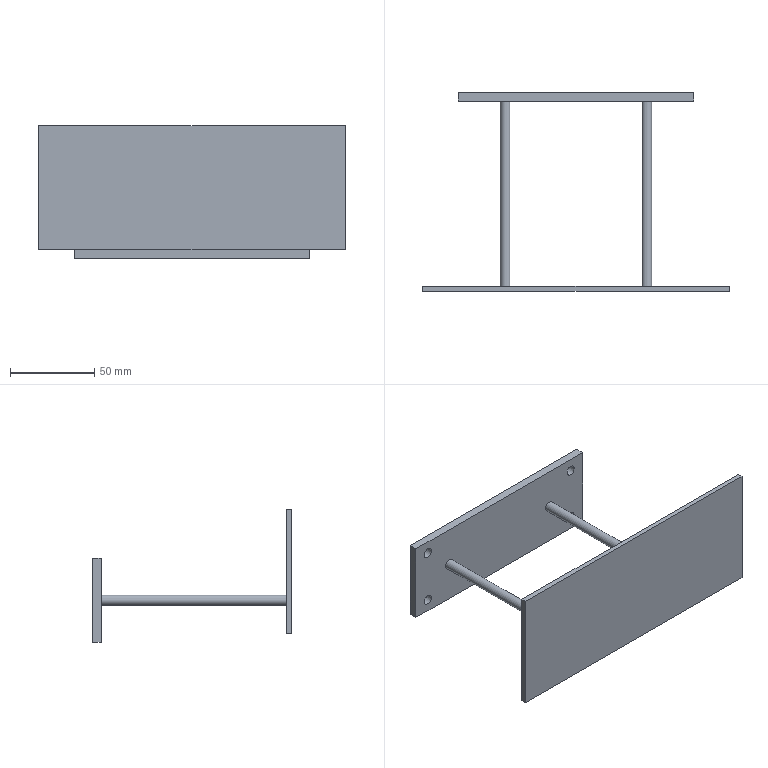Part | STEP file | zhijia2 | 1 solid | 18 faces | box 182 x 118 x 78.7 mm | volume 80895 mm3 | plane 12 | cylinder 6 | commonest cylinder face diameters 6 x6
STEP:
#1=CARTESIAN_POINT('',(0.,0.,0.));
#2=DIRECTION('',(0.,0.,1.));
#3=DIRECTION('',(1.,0.,0.));
#4=AXIS2_PLACEMENT_3D('',#1,#2,#3);
#5=CARTESIAN_POINT('',(-70.,-2.5,-25.));
#6=VERTEX_POINT('',#5);
#7=CARTESIAN_POINT('',(-70.,-2.5,25.));
#8=VERTEX_POINT('',#7);
#9=CARTESIAN_POINT('',(-70.,-2.5,-25.));
#10=DIRECTION('',(0.,0.,1.));
#11=VECTOR('',#10,1.);
#12=LINE('',#9,#11);
#13=CARTESIAN_POINT('',(-70.,2.5,-25.));
#14=DIRECTION('',(1.,0.,0.));
#15=DIRECTION('',(0.,0.,-1.));
#16=AXIS2_PLACEMENT_3D('',#13,#14,#15);
#17=PLANE('',#16);
#18=CARTESIAN_POINT('',(0.,-5.));
#19=DIRECTION('',(-1.,0.));
#20=VECTOR('',#19,1.);
#21=LINE('',#18,#20);
#22=(GEOMETRIC_REPRESENTATION_CONTEXT(2)PARAMETRIC_REPRESENTATION_CONTEXT()REPRESENTATION_CONTEXT('',''));
#23=DEFINITIONAL_REPRESENTATION('',(#21),#22);
#24=PCURVE('',#17,#23);
#25=CARTESIAN_POINT('',(0.,-2.5,0.));
#26=DIRECTION('',(0.,-1.,0.));
#27=DIRECTION('',(0.,0.,-1.));
#28=AXIS2_PLACEMENT_3D('',#25,#26,#27);
#29=PLANE('',#28);
#30=CARTESIAN_POINT('',(25.,-70.));
#31=DIRECTION('',(-1.,0.));
#32=VECTOR('',#31,1.);
#33=LINE('',#30,#32);
#34=(GEOMETRIC_REPRESENTATION_CONTEXT(2)PARAMETRIC_REPRESENTATION_CONTEXT()REPRESENTATION_CONTEXT('',''));
#35=DEFINITIONAL_REPRESENTATION('',(#33),#34);
#36=PCURVE('',#29,#35);
#37=SURFACE_CURVE('',#12,(#24,#36),.PCURVE_S1.);
#38=EDGE_CURVE('',#6,#8,#37,.T.);
#39=ORIENTED_EDGE('',*,*,#38,.T.);
#40=CARTESIAN_POINT('',(-70.,2.5,25.));
#41=VERTEX_POINT('',#40);
#42=CARTESIAN_POINT('',(-70.,2.5,25.));
#43=DIRECTION('',(0.,-1.,0.));
#44=VECTOR('',#43,1.);
#45=LINE('',#42,#44);
#46=CARTESIAN_POINT('',(-50.,0.));
#47=DIRECTION('',(0.,-1.));
#48=VECTOR('',#47,1.);
#49=LINE('',#46,#48);
#50=(GEOMETRIC_REPRESENTATION_CONTEXT(2)PARAMETRIC_REPRESENTATION_CONTEXT()REPRESENTATION_CONTEXT('',''));
#51=DEFINITIONAL_REPRESENTATION('',(#49),#50);
#52=PCURVE('',#17,#51);
#53=CARTESIAN_POINT('',(70.,2.5,25.));
#54=DIRECTION('',(0.,0.,-1.));
#55=DIRECTION('',(-1.,0.,0.));
#56=AXIS2_PLACEMENT_3D('',#53,#54,#55);
#57=PLANE('',#56);
#58=CARTESIAN_POINT('',(140.,0.));
#59=DIRECTION('',(0.,-1.));
#60=VECTOR('',#59,1.);
#61=LINE('',#58,#60);
#62=(GEOMETRIC_REPRESENTATION_CONTEXT(2)PARAMETRIC_REPRESENTATION_CONTEXT()REPRESENTATION_CONTEXT('',''));
#63=DEFINITIONAL_REPRESENTATION('',(#61),#62);
#64=PCURVE('',#57,#63);
#65=SURFACE_CURVE('',#45,(#52,#64),.PCURVE_S1.);
#66=EDGE_CURVE('',#41,#8,#65,.T.);
#67=ORIENTED_EDGE('',*,*,#66,.F.);
#68=CARTESIAN_POINT('',(-70.,2.5,-25.));
#69=VERTEX_POINT('',#68);
#70=CARTESIAN_POINT('',(-70.,2.5,-25.));
#71=DIRECTION('',(0.,0.,1.));
#72=VECTOR('',#71,1.);
#73=LINE('',#70,#72);
#74=CARTESIAN_POINT('',(0.,0.));
#75=DIRECTION('',(-1.,0.));
#76=VECTOR('',#75,1.);
#77=LINE('',#74,#76);
#78=(GEOMETRIC_REPRESENTATION_CONTEXT(2)PARAMETRIC_REPRESENTATION_CONTEXT()REPRESENTATION_CONTEXT('',''));
#79=DEFINITIONAL_REPRESENTATION('',(#77),#78);
#80=PCURVE('',#17,#79);
#81=CARTESIAN_POINT('',(0.,2.5,0.));
#82=DIRECTION('',(0.,-1.,0.));
#83=DIRECTION('',(0.,0.,-1.));
#84=AXIS2_PLACEMENT_3D('',#81,#82,#83);
#85=PLANE('',#84);
#86=CARTESIAN_POINT('',(25.,-70.));
#87=DIRECTION('',(-1.,0.));
#88=VECTOR('',#87,1.);
#89=LINE('',#86,#88);
#90=(GEOMETRIC_REPRESENTATION_CONTEXT(2)PARAMETRIC_REPRESENTATION_CONTEXT()REPRESENTATION_CONTEXT('',''));
#91=DEFINITIONAL_REPRESENTATION('',(#89),#90);
#92=PCURVE('',#85,#91);
#93=SURFACE_CURVE('',#73,(#80,#92),.PCURVE_S1.);
#94=EDGE_CURVE('',#69,#41,#93,.T.);
#95=ORIENTED_EDGE('',*,*,#94,.F.);
#96=CARTESIAN_POINT('',(-70.,2.5,-25.));
#97=DIRECTION('',(0.,-1.,0.));
#98=VECTOR('',#97,1.);
#99=LINE('',#96,#98);
#100=CARTESIAN_POINT('',(0.,0.));
#101=DIRECTION('',(0.,-1.));
#102=VECTOR('',#101,1.);
#103=LINE('',#100,#102);
#104=(GEOMETRIC_REPRESENTATION_CONTEXT(2)PARAMETRIC_REPRESENTATION_CONTEXT()REPRESENTATION_CONTEXT('',''));
#105=DEFINITIONAL_REPRESENTATION('',(#103),#104);
#106=PCURVE('',#17,#105);
#107=CARTESIAN_POINT('',(70.,2.5,-25.));
#108=DIRECTION('',(0.,0.,1.));
#109=DIRECTION('',(1.,0.,0.));
#110=AXIS2_PLACEMENT_3D('',#107,#108,#109);
#111=PLANE('',#110);
#112=CARTESIAN_POINT('',(-140.,0.));
#113=DIRECTION('',(0.,-1.));
#114=VECTOR('',#113,1.);
#115=LINE('',#112,#114);
#116=(GEOMETRIC_REPRESENTATION_CONTEXT(2)PARAMETRIC_REPRESENTATION_CONTEXT()REPRESENTATION_CONTEXT('',''));
#117=DEFINITIONAL_REPRESENTATION('',(#115),#116);
#118=PCURVE('',#111,#117);
#119=SURFACE_CURVE('',#99,(#106,#118),.PCURVE_S1.);
#120=EDGE_CURVE('',#69,#6,#119,.T.);
#121=ORIENTED_EDGE('',*,*,#120,.T.);
#122=EDGE_LOOP('',(#39,#67,#95,#121));
#123=FACE_BOUND('',#122,.T.);
#124=ADVANCED_FACE('',(#123),#17,.F.);
#125=CARTESIAN_POINT('',(70.,-2.5,25.));
#126=VERTEX_POINT('',#125);
#127=CARTESIAN_POINT('',(70.,-2.5,25.));
#128=DIRECTION('',(1.,0.,0.));
#129=VECTOR('',#128,1.);
#130=LINE('',#127,#129);
#131=CARTESIAN_POINT('',(0.,-5.));
#132=DIRECTION('',(-1.,0.));
#133=VECTOR('',#132,1.);
#134=LINE('',#131,#133);
#135=(GEOMETRIC_REPRESENTATION_CONTEXT(2)PARAMETRIC_REPRESENTATION_CONTEXT()REPRESENTATION_CONTEXT('',''));
#136=DEFINITIONAL_REPRESENTATION('',(#134),#135);
#137=PCURVE('',#57,#136);
#138=CARTESIAN_POINT('',(-25.,70.));
#139=DIRECTION('',(0.,1.));
#140=VECTOR('',#139,1.);
#141=LINE('',#138,#140);
#142=(GEOMETRIC_REPRESENTATION_CONTEXT(2)PARAMETRIC_REPRESENTATION_CONTEXT()REPRESENTATION_CONTEXT('',''));
#143=DEFINITIONAL_REPRESENTATION('',(#141),#142);
#144=PCURVE('',#29,#143);
#145=SURFACE_CURVE('',#130,(#137,#144),.PCURVE_S1.);
#146=EDGE_CURVE('',#8,#126,#145,.T.);
#147=ORIENTED_EDGE('',*,*,#146,.T.);
#148=CARTESIAN_POINT('',(70.,2.5,25.));
#149=VERTEX_POINT('',#148);
#150=CARTESIAN_POINT('',(70.,2.5,25.));
#151=DIRECTION('',(0.,-1.,0.));
#152=VECTOR('',#151,1.);
#153=LINE('',#150,#152);
#154=CARTESIAN_POINT('',(0.,0.));
#155=DIRECTION('',(0.,-1.));
#156=VECTOR('',#155,1.);
#157=LINE('',#154,#156);
#158=(GEOMETRIC_REPRESENTATION_CONTEXT(2)PARAMETRIC_REPRESENTATION_CONTEXT()REPRESENTATION_CONTEXT('',''));
#159=DEFINITIONAL_REPRESENTATION('',(#157),#158);
#160=PCURVE('',#57,#159);
#161=CARTESIAN_POINT('',(70.,2.5,-25.));
#162=DIRECTION('',(-1.,0.,0.));
#163=DIRECTION('',(0.,0.,1.));
#164=AXIS2_PLACEMENT_3D('',#161,#162,#163);
#165=PLANE('',#164);
#166=CARTESIAN_POINT('',(50.,0.));
#167=DIRECTION('',(0.,-1.));
#168=VECTOR('',#167,1.);
#169=LINE('',#166,#168);
#170=(GEOMETRIC_REPRESENTATION_CONTEXT(2)PARAMETRIC_REPRESENTATION_CONTEXT()REPRESENTATION_CONTEXT('',''));
#171=DEFINITIONAL_REPRESENTATION('',(#169),#170);
#172=PCURVE('',#165,#171);
#173=SURFACE_CURVE('',#153,(#160,#172),.PCURVE_S1.);
#174=EDGE_CURVE('',#149,#126,#173,.T.);
#175=ORIENTED_EDGE('',*,*,#174,.F.);
#176=CARTESIAN_POINT('',(70.,2.5,25.));
#177=DIRECTION('',(1.,0.,0.));
#178=VECTOR('',#177,1.);
#179=LINE('',#176,#178);
#180=CARTESIAN_POINT('',(0.,0.));
#181=DIRECTION('',(-1.,0.));
#182=VECTOR('',#181,1.);
#183=LINE('',#180,#182);
#184=(GEOMETRIC_REPRESENTATION_CONTEXT(2)PARAMETRIC_REPRESENTATION_CONTEXT()REPRESENTATION_CONTEXT('',''));
#185=DEFINITIONAL_REPRESENTATION('',(#183),#184);
#186=PCURVE('',#57,#185);
#187=CARTESIAN_POINT('',(-25.,70.));
#188=DIRECTION('',(0.,1.));
#189=VECTOR('',#188,1.);
#190=LINE('',#187,#189);
#191=(GEOMETRIC_REPRESENTATION_CONTEXT(2)PARAMETRIC_REPRESENTATION_CONTEXT()REPRESENTATION_CONTEXT('',''));
#192=DEFINITIONAL_REPRESENTATION('',(#190),#191);
#193=PCURVE('',#85,#192);
#194=SURFACE_CURVE('',#179,(#186,#193),.PCURVE_S1.);
#195=EDGE_CURVE('',#41,#149,#194,.T.);
#196=ORIENTED_EDGE('',*,*,#195,.F.);
#197=ORIENTED_EDGE('',*,*,#66,.T.);
#198=EDGE_LOOP('',(#147,#175,#196,#197));
#199=FACE_BOUND('',#198,.T.);
#200=ADVANCED_FACE('',(#199),#57,.F.);
#201=CARTESIAN_POINT('',(70.,-2.5,-25.));
#202=VERTEX_POINT('',#201);
#203=CARTESIAN_POINT('',(70.,-2.5,-25.));
#204=DIRECTION('',(0.,0.,-1.));
#205=VECTOR('',#204,1.);
#206=LINE('',#203,#205);
#207=CARTESIAN_POINT('',(0.,-5.));
#208=DIRECTION('',(-1.,0.));
#209=VECTOR('',#208,1.);
#210=LINE('',#207,#209);
#211=(GEOMETRIC_REPRESENTATION_CONTEXT(2)PARAMETRIC_REPRESENTATION_CONTEXT()REPRESENTATION_CONTEXT('',''));
#212=DEFINITIONAL_REPRESENTATION('',(#210),#211);
#213=PCURVE('',#165,#212);
#214=CARTESIAN_POINT('',(25.,70.));
#215=DIRECTION('',(1.,0.));
#216=VECTOR('',#215,1.);
#217=LINE('',#214,#216);
#218=(GEOMETRIC_REPRESENTATION_CONTEXT(2)PARAMETRIC_REPRESENTATION_CONTEXT()REPRESENTATION_CONTEXT('',''));
#219=DEFINITIONAL_REPRESENTATION('',(#217),#218);
#220=PCURVE('',#29,#219);
#221=SURFACE_CURVE('',#206,(#213,#220),.PCURVE_S1.);
#222=EDGE_CURVE('',#126,#202,#221,.T.);
#223=ORIENTED_EDGE('',*,*,#222,.T.);
#224=CARTESIAN_POINT('',(70.,2.5,-25.));
#225=VERTEX_POINT('',#224);
#226=CARTESIAN_POINT('',(70.,2.5,-25.));
#227=DIRECTION('',(0.,-1.,0.));
#228=VECTOR('',#227,1.);
#229=LINE('',#226,#228);
#230=CARTESIAN_POINT('',(0.,0.));
#231=DIRECTION('',(0.,-1.));
#232=VECTOR('',#231,1.);
#233=LINE('',#230,#232);
#234=(GEOMETRIC_REPRESENTATION_CONTEXT(2)PARAMETRIC_REPRESENTATION_CONTEXT()REPRESENTATION_CONTEXT('',''));
#235=DEFINITIONAL_REPRESENTATION('',(#233),#234);
#236=PCURVE('',#165,#235);
#237=CARTESIAN_POINT('',(0.,0.));
#238=DIRECTION('',(0.,-1.));
#239=VECTOR('',#238,1.);
#240=LINE('',#237,#239);
#241=(GEOMETRIC_REPRESENTATION_CONTEXT(2)PARAMETRIC_REPRESENTATION_CONTEXT()REPRESENTATION_CONTEXT('',''));
#242=DEFINITIONAL_REPRESENTATION('',(#240),#241);
#243=PCURVE('',#111,#242);
#244=SURFACE_CURVE('',#229,(#236,#243),.PCURVE_S1.);
#245=EDGE_CURVE('',#225,#202,#244,.T.);
#246=ORIENTED_EDGE('',*,*,#245,.F.);
#247=CARTESIAN_POINT('',(70.,2.5,-25.));
#248=DIRECTION('',(0.,0.,-1.));
#249=VECTOR('',#248,1.);
#250=LINE('',#247,#249);
#251=CARTESIAN_POINT('',(0.,0.));
#252=DIRECTION('',(-1.,0.));
#253=VECTOR('',#252,1.);
#254=LINE('',#251,#253);
#255=(GEOMETRIC_REPRESENTATION_CONTEXT(2)PARAMETRIC_REPRESENTATION_CONTEXT()REPRESENTATION_CONTEXT('',''));
#256=DEFINITIONAL_REPRESENTATION('',(#254),#255);
#257=PCURVE('',#165,#256);
#258=CARTESIAN_POINT('',(25.,70.));
#259=DIRECTION('',(1.,0.));
#260=VECTOR('',#259,1.);
#261=LINE('',#258,#260);
#262=(GEOMETRIC_REPRESENTATION_CONTEXT(2)PARAMETRIC_REPRESENTATION_CONTEXT()REPRESENTATION_CONTEXT('',''));
#263=DEFINITIONAL_REPRESENTATION('',(#261),#262);
#264=PCURVE('',#85,#263);
#265=SURFACE_CURVE('',#250,(#257,#264),.PCURVE_S1.);
#266=EDGE_CURVE('',#149,#225,#265,.T.);
#267=ORIENTED_EDGE('',*,*,#266,.F.);
#268=ORIENTED_EDGE('',*,*,#174,.T.);
#269=EDGE_LOOP('',(#223,#246,#267,#268));
#270=FACE_BOUND('',#269,.T.);
#271=ADVANCED_FACE('',(#270),#165,.F.);
#272=CARTESIAN_POINT('',(70.,-2.5,-25.));
#273=DIRECTION('',(-1.,0.,0.));
#274=VECTOR('',#273,1.);
#275=LINE('',#272,#274);
#276=CARTESIAN_POINT('',(0.,-5.));
#277=DIRECTION('',(-1.,0.));
#278=VECTOR('',#277,1.);
#279=LINE('',#276,#278);
#280=(GEOMETRIC_REPRESENTATION_CONTEXT(2)PARAMETRIC_REPRESENTATION_CONTEXT()REPRESENTATION_CONTEXT('',''));
#281=DEFINITIONAL_REPRESENTATION('',(#279),#280);
#282=PCURVE('',#111,#281);
#283=CARTESIAN_POINT('',(25.,70.));
#284=DIRECTION('',(0.,-1.));
#285=VECTOR('',#284,1.);
#286=LINE('',#283,#285);
#287=(GEOMETRIC_REPRESENTATION_CONTEXT(2)PARAMETRIC_REPRESENTATION_CONTEXT()REPRESENTATION_CONTEXT('',''));
#288=DEFINITIONAL_REPRESENTATION('',(#286),#287);
#289=PCURVE('',#29,#288);
#290=SURFACE_CURVE('',#275,(#282,#289),.PCURVE_S1.);
#291=EDGE_CURVE('',#202,#6,#290,.T.);
#292=ORIENTED_EDGE('',*,*,#291,.T.);
#293=ORIENTED_EDGE('',*,*,#120,.F.);
#294=CARTESIAN_POINT('',(70.,2.5,-25.));
#295=DIRECTION('',(-1.,0.,0.));
#296=VECTOR('',#295,1.);
#297=LINE('',#294,#296);
#298=CARTESIAN_POINT('',(0.,0.));
#299=DIRECTION('',(-1.,0.));
#300=VECTOR('',#299,1.);
#301=LINE('',#298,#300);
#302=(GEOMETRIC_REPRESENTATION_CONTEXT(2)PARAMETRIC_REPRESENTATION_CONTEXT()REPRESENTATION_CONTEXT('',''));
#303=DEFINITIONAL_REPRESENTATION('',(#301),#302);
#304=PCURVE('',#111,#303);
#305=CARTESIAN_POINT('',(25.,70.));
#306=DIRECTION('',(0.,-1.));
#307=VECTOR('',#306,1.);
#308=LINE('',#305,#307);
#309=(GEOMETRIC_REPRESENTATION_CONTEXT(2)PARAMETRIC_REPRESENTATION_CONTEXT()REPRESENTATION_CONTEXT('',''));
#310=DEFINITIONAL_REPRESENTATION('',(#308),#309);
#311=PCURVE('',#85,#310);
#312=SURFACE_CURVE('',#297,(#304,#311),.PCURVE_S1.);
#313=EDGE_CURVE('',#225,#69,#312,.T.);
#314=ORIENTED_EDGE('',*,*,#313,.F.);
#315=ORIENTED_EDGE('',*,*,#245,.T.);
#316=EDGE_LOOP('',(#292,#293,#314,#315));
#317=FACE_BOUND('',#316,.T.);
#318=ADVANCED_FACE('',(#317),#111,.F.);
#319=CARTESIAN_POINT('',(-60.,2.5,20.));
#320=VERTEX_POINT('',#319);
#321=CARTESIAN_POINT('',(-60.,2.5,17.));
#322=DIRECTION('',(0.,1.,0.));
#323=DIRECTION('',(0.,0.,1.));
#324=AXIS2_PLACEMENT_3D('',#321,#322,#323);
#325=CIRCLE('',#324,3.);
#326=CARTESIAN_POINT('',(-20.,-60.));
#327=CARTESIAN_POINT('',(-20.,-54.804));
#328=CARTESIAN_POINT('',(-15.5,-57.402));
#329=CARTESIAN_POINT('',(-11.,-60.));
#330=CARTESIAN_POINT('',(-15.5,-62.598));
#331=CARTESIAN_POINT('',(-20.,-65.196));
#332=CARTESIAN_POINT('',(-20.,-60.));
#333=(BOUNDED_CURVE()B_SPLINE_CURVE(2,(#326,#327,#328,#329,#330,#331,#332),.UNSPECIFIED.,.T.,.F.)B_SPLINE_CURVE_WITH_KNOTS((1,2,2,2,2,1),(-2.094,0.,2.094,4.189,6.283,8.378),.UNSPECIFIED.)CURVE()GEOMETRIC_REPRESENTATION_ITEM()RATIONAL_B_SPLINE_CURVE((1.,0.5,1.,0.5,1.,0.5,1.))REPRESENTATION_ITEM(''));
#334=(GEOMETRIC_REPRESENTATION_CONTEXT(2)PARAMETRIC_REPRESENTATION_CONTEXT()REPRESENTATION_CONTEXT('',''));
#335=DEFINITIONAL_REPRESENTATION('',(#333),#334);
#336=PCURVE('',#85,#335);
#337=CARTESIAN_POINT('',(-60.,-2.5,17.));
#338=DIRECTION('',(0.,1.,0.));
#339=DIRECTION('',(0.,0.,1.));
#340=AXIS2_PLACEMENT_3D('',#337,#338,#339);
#341=CYLINDRICAL_SURFACE('',#340,3.);
#342=CARTESIAN_POINT('',(0.,5.));
#343=DIRECTION('',(1.,0.));
#344=VECTOR('',#343,1.);
#345=LINE('',#342,#344);
#346=(GEOMETRIC_REPRESENTATION_CONTEXT(2)PARAMETRIC_REPRESENTATION_CONTEXT()REPRESENTATION_CONTEXT('',''));
#347=DEFINITIONAL_REPRESENTATION('',(#345),#346);
#348=PCURVE('',#341,#347);
#349=SURFACE_CURVE('',#325,(#336,#348),.PCURVE_S1.);
#350=EDGE_CURVE('',#320,#320,#349,.T.);
#351=ORIENTED_EDGE('',*,*,#350,.F.);
#352=EDGE_LOOP('',(#351));
#353=FACE_BOUND('',#352,.T.);
#354=CARTESIAN_POINT('',(60.,2.5,14.));
#355=VERTEX_POINT('',#354);
#356=CARTESIAN_POINT('',(60.,2.5,17.));
#357=DIRECTION('',(0.,1.,0.));
#358=DIRECTION('',(0.,0.,-1.));
#359=AXIS2_PLACEMENT_3D('',#356,#357,#358);
#360=CIRCLE('',#359,3.);
#361=CARTESIAN_POINT('',(-14.,60.));
#362=CARTESIAN_POINT('',(-14.,54.804));
#363=CARTESIAN_POINT('',(-18.5,57.402));
#364=CARTESIAN_POINT('',(-23.,60.));
#365=CARTESIAN_POINT('',(-18.5,62.598));
#366=CARTESIAN_POINT('',(-14.,65.196));
#367=CARTESIAN_POINT('',(-14.,60.));
#368=(BOUNDED_CURVE()B_SPLINE_CURVE(2,(#361,#362,#363,#364,#365,#366,#367),.UNSPECIFIED.,.T.,.F.)B_SPLINE_CURVE_WITH_KNOTS((1,2,2,2,2,1),(-2.094,0.,2.094,4.189,6.283,8.378),.UNSPECIFIED.)CURVE()GEOMETRIC_REPRESENTATION_ITEM()RATIONAL_B_SPLINE_CURVE((1.,0.5,1.,0.5,1.,0.5,1.))REPRESENTATION_ITEM(''));
#369=(GEOMETRIC_REPRESENTATION_CONTEXT(2)PARAMETRIC_REPRESENTATION_CONTEXT()REPRESENTATION_CONTEXT('',''));
#370=DEFINITIONAL_REPRESENTATION('',(#368),#369);
#371=PCURVE('',#85,#370);
#372=CARTESIAN_POINT('',(60.,-2.5,17.));
#373=DIRECTION('',(0.,1.,0.));
#374=DIRECTION('',(0.,0.,1.));
#375=AXIS2_PLACEMENT_3D('',#372,#373,#374);
#376=CYLINDRICAL_SURFACE('',#375,3.);
#377=CARTESIAN_POINT('',(3.142,5.));
#378=DIRECTION('',(1.,0.));
#379=VECTOR('',#378,1.);
#380=LINE('',#377,#379);
#381=(GEOMETRIC_REPRESENTATION_CONTEXT(2)PARAMETRIC_REPRESENTATION_CONTEXT()REPRESENTATION_CONTEXT('',''));
#382=DEFINITIONAL_REPRESENTATION('',(#380),#381);
#383=PCURVE('',#376,#382);
#384=SURFACE_CURVE('',#360,(#371,#383),.PCURVE_S1.);
#385=EDGE_CURVE('',#355,#355,#384,.T.);
#386=ORIENTED_EDGE('',*,*,#385,.F.);
#387=EDGE_LOOP('',(#386));
#388=FACE_BOUND('',#387,.T.);
#389=CARTESIAN_POINT('',(60.,2.5,-20.));
#390=VERTEX_POINT('',#389);
#391=CARTESIAN_POINT('',(60.,2.5,-17.));
#392=DIRECTION('',(0.,1.,0.));
#393=DIRECTION('',(0.,0.,-1.));
#394=AXIS2_PLACEMENT_3D('',#391,#392,#393);
#395=CIRCLE('',#394,3.);
#396=CARTESIAN_POINT('',(20.,60.));
#397=CARTESIAN_POINT('',(20.,54.804));
#398=CARTESIAN_POINT('',(15.5,57.402));
#399=CARTESIAN_POINT('',(11.,60.));
#400=CARTESIAN_POINT('',(15.5,62.598));
#401=CARTESIAN_POINT('',(20.,65.196));
#402=CARTESIAN_POINT('',(20.,60.));
#403=(BOUNDED_CURVE()B_SPLINE_CURVE(2,(#396,#397,#398,#399,#400,#401,#402),.UNSPECIFIED.,.T.,.F.)B_SPLINE_CURVE_WITH_KNOTS((1,2,2,2,2,1),(-2.094,0.,2.094,4.189,6.283,8.378),.UNSPECIFIED.)CURVE()GEOMETRIC_REPRESENTATION_ITEM()RATIONAL_B_SPLINE_CURVE((1.,0.5,1.,0.5,1.,0.5,1.))REPRESENTATION_ITEM(''));
#404=(GEOMETRIC_REPRESENTATION_CONTEXT(2)PARAMETRIC_REPRESENTATION_CONTEXT()REPRESENTATION_CONTEXT('',''));
#405=DEFINITIONAL_REPRESENTATION('',(#403),#404);
#406=PCURVE('',#85,#405);
#407=CARTESIAN_POINT('',(60.,-2.5,-17.));
#408=DIRECTION('',(0.,1.,0.));
#409=DIRECTION('',(0.,0.,1.));
#410=AXIS2_PLACEMENT_3D('',#407,#408,#409);
#411=CYLINDRICAL_SURFACE('',#410,3.);
#412=CARTESIAN_POINT('',(3.142,5.));
#413=DIRECTION('',(1.,0.));
#414=VECTOR('',#413,1.);
#415=LINE('',#412,#414);
#416=(GEOMETRIC_REPRESENTATION_CONTEXT(2)PARAMETRIC_REPRESENTATION_CONTEXT()REPRESENTATION_CONTEXT('',''));
#417=DEFINITIONAL_REPRESENTATION('',(#415),#416);
#418=PCURVE('',#411,#417);
#419=SURFACE_CURVE('',#395,(#406,#418),.PCURVE_S1.);
#420=EDGE_CURVE('',#390,#390,#419,.T.);
#421=ORIENTED_EDGE('',*,*,#420,.F.);
#422=EDGE_LOOP('',(#421));
#423=FACE_BOUND('',#422,.T.);
#424=CARTESIAN_POINT('',(-60.,2.5,-14.));
#425=VERTEX_POINT('',#424);
#426=CARTESIAN_POINT('',(-60.,2.5,-17.));
#427=DIRECTION('',(0.,1.,0.));
#428=DIRECTION('',(0.,0.,1.));
#429=AXIS2_PLACEMENT_3D('',#426,#427,#428);
#430=CIRCLE('',#429,3.);
#431=CARTESIAN_POINT('',(14.,-60.));
#432=CARTESIAN_POINT('',(14.,-54.804));
#433=CARTESIAN_POINT('',(18.5,-57.402));
#434=CARTESIAN_POINT('',(23.,-60.));
#435=CARTESIAN_POINT('',(18.5,-62.598));
#436=CARTESIAN_POINT('',(14.,-65.196));
#437=CARTESIAN_POINT('',(14.,-60.));
#438=(BOUNDED_CURVE()B_SPLINE_CURVE(2,(#431,#432,#433,#434,#435,#436,#437),.UNSPECIFIED.,.T.,.F.)B_SPLINE_CURVE_WITH_KNOTS((1,2,2,2,2,1),(-2.094,0.,2.094,4.189,6.283,8.378),.UNSPECIFIED.)CURVE()GEOMETRIC_REPRESENTATION_ITEM()RATIONAL_B_SPLINE_CURVE((1.,0.5,1.,0.5,1.,0.5,1.))REPRESENTATION_ITEM(''));
#439=(GEOMETRIC_REPRESENTATION_CONTEXT(2)PARAMETRIC_REPRESENTATION_CONTEXT()REPRESENTATION_CONTEXT('',''));
#440=DEFINITIONAL_REPRESENTATION('',(#438),#439);
#441=PCURVE('',#85,#440);
#442=CARTESIAN_POINT('',(-60.,-2.5,-17.));
#443=DIRECTION('',(0.,1.,0.));
#444=DIRECTION('',(0.,0.,1.));
#445=AXIS2_PLACEMENT_3D('',#442,#443,#444);
#446=CYLINDRICAL_SURFACE('',#445,3.);
#447=CARTESIAN_POINT('',(0.,5.));
#448=DIRECTION('',(1.,0.));
#449=VECTOR('',#448,1.);
#450=LINE('',#447,#449);
#451=(GEOMETRIC_REPRESENTATION_CONTEXT(2)PARAMETRIC_REPRESENTATION_CONTEXT()REPRESENTATION_CONTEXT('',''));
#452=DEFINITIONAL_REPRESENTATION('',(#450),#451);
#453=PCURVE('',#446,#452);
#454=SURFACE_CURVE('',#430,(#441,#453),.PCURVE_S1.);
#455=EDGE_CURVE('',#425,#425,#454,.T.);
#456=ORIENTED_EDGE('',*,*,#455,.F.);
#457=EDGE_LOOP('',(#456));
#458=FACE_BOUND('',#457,.T.);
#459=ORIENTED_EDGE('',*,*,#94,.T.);
#460=ORIENTED_EDGE('',*,*,#195,.T.);
#461=ORIENTED_EDGE('',*,*,#266,.T.);
#462=ORIENTED_EDGE('',*,*,#313,.T.);
#463=EDGE_LOOP('',(#459,#460,#461,#462));
#464=FACE_BOUND('',#463,.T.);
#465=ADVANCED_FACE('',(#353,#388,#423,#458,#464),#85,.F.);
#466=CARTESIAN_POINT('',(42.,-2.5,3.));
#467=VERTEX_POINT('',#466);
#468=CARTESIAN_POINT('',(42.,-2.5,0.));
#469=DIRECTION('',(0.,-1.,0.));
#470=DIRECTION('',(0.,0.,1.));
#471=AXIS2_PLACEMENT_3D('',#468,#469,#470);
#472=CIRCLE('',#471,3.);
#473=CARTESIAN_POINT('',(0.,42.));
#474=DIRECTION('',(-1.,0.));
#475=AXIS2_PLACEMENT_2D('',#473,#474);
#476=CIRCLE('',#475,3.);
#477=(GEOMETRIC_REPRESENTATION_CONTEXT(2)PARAMETRIC_REPRESENTATION_CONTEXT()REPRESENTATION_CONTEXT('',''));
#478=DEFINITIONAL_REPRESENTATION('',(#476),#477);
#479=PCURVE('',#29,#478);
#480=CARTESIAN_POINT('',(42.,-112.5,0.));
#481=DIRECTION('',(0.,1.,0.));
#482=DIRECTION('',(0.,0.,1.));
#483=AXIS2_PLACEMENT_3D('',#480,#481,#482);
#484=CYLINDRICAL_SURFACE('',#483,3.);
#485=CARTESIAN_POINT('',(6.283,110.));
#486=DIRECTION('',(-1.,0.));
#487=VECTOR('',#486,1.);
#488=LINE('',#485,#487);
#489=(GEOMETRIC_REPRESENTATION_CONTEXT(2)PARAMETRIC_REPRESENTATION_CONTEXT()REPRESENTATION_CONTEXT('',''));
#490=DEFINITIONAL_REPRESENTATION('',(#488),#489);
#491=PCURVE('',#484,#490);
#492=SURFACE_CURVE('',#472,(#479,#491),.PCURVE_S1.);
#493=EDGE_CURVE('',#467,#467,#492,.T.);
#494=ORIENTED_EDGE('',*,*,#493,.F.);
#495=EDGE_LOOP('',(#494));
#496=FACE_BOUND('',#495,.T.);
#497=CARTESIAN_POINT('',(-42.,-2.5,-3.));
#498=VERTEX_POINT('',#497);
#499=CARTESIAN_POINT('',(-42.,-2.5,0.));
#500=DIRECTION('',(0.,-1.,0.));
#501=DIRECTION('',(0.,0.,-1.));
#502=AXIS2_PLACEMENT_3D('',#499,#500,#501);
#503=CIRCLE('',#502,3.);
#504=CARTESIAN_POINT('',(0.,-42.));
#505=DIRECTION('',(1.,0.));
#506=AXIS2_PLACEMENT_2D('',#504,#505);
#507=CIRCLE('',#506,3.);
#508=(GEOMETRIC_REPRESENTATION_CONTEXT(2)PARAMETRIC_REPRESENTATION_CONTEXT()REPRESENTATION_CONTEXT('',''));
#509=DEFINITIONAL_REPRESENTATION('',(#507),#508);
#510=PCURVE('',#29,#509);
#511=CARTESIAN_POINT('',(-42.,-112.5,0.));
#512=DIRECTION('',(0.,1.,0.));
#513=DIRECTION('',(0.,0.,1.));
#514=AXIS2_PLACEMENT_3D('',#511,#512,#513);
#515=CYLINDRICAL_SURFACE('',#514,3.);
#516=CARTESIAN_POINT('',(9.425,110.));
#517=DIRECTION('',(-1.,0.));
#518=VECTOR('',#517,1.);
#519=LINE('',#516,#518);
#520=(GEOMETRIC_REPRESENTATION_CONTEXT(2)PARAMETRIC_REPRESENTATION_CONTEXT()REPRESENTATION_CONTEXT('',''));
#521=DEFINITIONAL_REPRESENTATION('',(#519),#520);
#522=PCURVE('',#515,#521);
#523=SURFACE_CURVE('',#503,(#510,#522),.PCURVE_S1.);
#524=EDGE_CURVE('',#498,#498,#523,.T.);
#525=ORIENTED_EDGE('',*,*,#524,.F.);
#526=EDGE_LOOP('',(#525));
#527=FACE_BOUND('',#526,.T.);
#528=CARTESIAN_POINT('',(-60.,-2.5,20.));
#529=VERTEX_POINT('',#528);
#530=CARTESIAN_POINT('',(-60.,-2.5,17.));
#531=DIRECTION('',(0.,1.,0.));
#532=DIRECTION('',(0.,0.,1.));
#533=AXIS2_PLACEMENT_3D('',#530,#531,#532);
#534=CIRCLE('',#533,3.);
#535=CARTESIAN_POINT('',(-20.,-60.));
#536=CARTESIAN_POINT('',(-20.,-54.804));
#537=CARTESIAN_POINT('',(-15.5,-57.402));
#538=CARTESIAN_POINT('',(-11.,-60.));
#539=CARTESIAN_POINT('',(-15.5,-62.598));
#540=CARTESIAN_POINT('',(-20.,-65.196));
#541=CARTESIAN_POINT('',(-20.,-60.));
#542=(BOUNDED_CURVE()B_SPLINE_CURVE(2,(#535,#536,#537,#538,#539,#540,#541),.UNSPECIFIED.,.T.,.F.)B_SPLINE_CURVE_WITH_KNOTS((1,2,2,2,2,1),(-2.094,0.,2.094,4.189,6.283,8.378),.UNSPECIFIED.)CURVE()GEOMETRIC_REPRESENTATION_ITEM()RATIONAL_B_SPLINE_CURVE((1.,0.5,1.,0.5,1.,0.5,1.))REPRESENTATION_ITEM(''));
#543=(GEOMETRIC_REPRESENTATION_CONTEXT(2)PARAMETRIC_REPRESENTATION_CONTEXT()REPRESENTATION_CONTEXT('',''));
#544=DEFINITIONAL_REPRESENTATION('',(#542),#543);
#545=PCURVE('',#29,#544);
#546=CARTESIAN_POINT('',(0.,0.));
#547=DIRECTION('',(1.,0.));
#548=VECTOR('',#547,1.);
#549=LINE('',#546,#548);
#550=(GEOMETRIC_REPRESENTATION_CONTEXT(2)PARAMETRIC_REPRESENTATION_CONTEXT()REPRESENTATION_CONTEXT('',''));
#551=DEFINITIONAL_REPRESENTATION('',(#549),#550);
#552=PCURVE('',#341,#551);
#553=SURFACE_CURVE('',#534,(#545,#552),.PCURVE_S1.);
#554=EDGE_CURVE('',#529,#529,#553,.T.);
#555=ORIENTED_EDGE('',*,*,#554,.T.);
#556=EDGE_LOOP('',(#555));
#557=FACE_BOUND('',#556,.T.);
#558=CARTESIAN_POINT('',(60.,-2.5,14.));
#559=VERTEX_POINT('',#558);
#560=CARTESIAN_POINT('',(60.,-2.5,17.));
#561=DIRECTION('',(0.,1.,0.));
#562=DIRECTION('',(0.,0.,-1.));
#563=AXIS2_PLACEMENT_3D('',#560,#561,#562);
#564=CIRCLE('',#563,3.);
#565=CARTESIAN_POINT('',(-14.,60.));
#566=CARTESIAN_POINT('',(-14.,54.804));
#567=CARTESIAN_POINT('',(-18.5,57.402));
#568=CARTESIAN_POINT('',(-23.,60.));
#569=CARTESIAN_POINT('',(-18.5,62.598));
#570=CARTESIAN_POINT('',(-14.,65.196));
#571=CARTESIAN_POINT('',(-14.,60.));
#572=(BOUNDED_CURVE()B_SPLINE_CURVE(2,(#565,#566,#567,#568,#569,#570,#571),.UNSPECIFIED.,.T.,.F.)B_SPLINE_CURVE_WITH_KNOTS((1,2,2,2,2,1),(-2.094,0.,2.094,4.189,6.283,8.378),.UNSPECIFIED.)CURVE()GEOMETRIC_REPRESENTATION_ITEM()RATIONAL_B_SPLINE_CURVE((1.,0.5,1.,0.5,1.,0.5,1.))REPRESENTATION_ITEM(''));
#573=(GEOMETRIC_REPRESENTATION_CONTEXT(2)PARAMETRIC_REPRESENTATION_CONTEXT()REPRESENTATION_CONTEXT('',''));
#574=DEFINITIONAL_REPRESENTATION('',(#572),#573);
#575=PCURVE('',#29,#574);
#576=CARTESIAN_POINT('',(3.142,0.));
#577=DIRECTION('',(1.,0.));
#578=VECTOR('',#577,1.);
#579=LINE('',#576,#578);
#580=(GEOMETRIC_REPRESENTATION_CONTEXT(2)PARAMETRIC_REPRESENTATION_CONTEXT()REPRESENTATION_CONTEXT('',''));
#581=DEFINITIONAL_REPRESENTATION('',(#579),#580);
#582=PCURVE('',#376,#581);
#583=SURFACE_CURVE('',#564,(#575,#582),.PCURVE_S1.);
#584=EDGE_CURVE('',#559,#559,#583,.T.);
#585=ORIENTED_EDGE('',*,*,#584,.T.);
#586=EDGE_LOOP('',(#585));
#587=FACE_BOUND('',#586,.T.);
#588=CARTESIAN_POINT('',(60.,-2.5,-20.));
#589=VERTEX_POINT('',#588);
#590=CARTESIAN_POINT('',(60.,-2.5,-17.));
#591=DIRECTION('',(0.,1.,0.));
#592=DIRECTION('',(0.,0.,-1.));
#593=AXIS2_PLACEMENT_3D('',#590,#591,#592);
#594=CIRCLE('',#593,3.);
#595=CARTESIAN_POINT('',(20.,60.));
#596=CARTESIAN_POINT('',(20.,54.804));
#597=CARTESIAN_POINT('',(15.5,57.402));
#598=CARTESIAN_POINT('',(11.,60.));
#599=CARTESIAN_POINT('',(15.5,62.598));
#600=CARTESIAN_POINT('',(20.,65.196));
#601=CARTESIAN_POINT('',(20.,60.));
#602=(BOUNDED_CURVE()B_SPLINE_CURVE(2,(#595,#596,#597,#598,#599,#600,#601),.UNSPECIFIED.,.T.,.F.)B_SPLINE_CURVE_WITH_KNOTS((1,2,2,2,2,1),(-2.094,0.,2.094,4.189,6.283,8.378),.UNSPECIFIED.)CURVE()GEOMETRIC_REPRESENTATION_ITEM()RATIONAL_B_SPLINE_CURVE((1.,0.5,1.,0.5,1.,0.5,1.))REPRESENTATION_ITEM(''));
#603=(GEOMETRIC_REPRESENTATION_CONTEXT(2)PARAMETRIC_REPRESENTATION_CONTEXT()REPRESENTATION_CONTEXT('',''));
#604=DEFINITIONAL_REPRESENTATION('',(#602),#603);
#605=PCURVE('',#29,#604);
#606=CARTESIAN_POINT('',(3.142,0.));
#607=DIRECTION('',(1.,0.));
#608=VECTOR('',#607,1.);
#609=LINE('',#606,#608);
#610=(GEOMETRIC_REPRESENTATION_CONTEXT(2)PARAMETRIC_REPRESENTATION_CONTEXT()REPRESENTATION_CONTEXT('',''));
#611=DEFINITIONAL_REPRESENTATION('',(#609),#610);
#612=PCURVE('',#411,#611);
#613=SURFACE_CURVE('',#594,(#605,#612),.PCURVE_S1.);
#614=EDGE_CURVE('',#589,#589,#613,.T.);
#615=ORIENTED_EDGE('',*,*,#614,.T.);
#616=EDGE_LOOP('',(#615));
#617=FACE_BOUND('',#616,.T.);
#618=CARTESIAN_POINT('',(-60.,-2.5,-14.));
#619=VERTEX_POINT('',#618);
#620=CARTESIAN_POINT('',(-60.,-2.5,-17.));
#621=DIRECTION('',(0.,1.,0.));
#622=DIRECTION('',(0.,0.,1.));
#623=AXIS2_PLACEMENT_3D('',#620,#621,#622);
#624=CIRCLE('',#623,3.);
#625=CARTESIAN_POINT('',(14.,-60.));
#626=CARTESIAN_POINT('',(14.,-54.804));
#627=CARTESIAN_POINT('',(18.5,-57.402));
#628=CARTESIAN_POINT('',(23.,-60.));
#629=CARTESIAN_POINT('',(18.5,-62.598));
#630=CARTESIAN_POINT('',(14.,-65.196));
#631=CARTESIAN_POINT('',(14.,-60.));
#632=(BOUNDED_CURVE()B_SPLINE_CURVE(2,(#625,#626,#627,#628,#629,#630,#631),.UNSPECIFIED.,.T.,.F.)B_SPLINE_CURVE_WITH_KNOTS((1,2,2,2,2,1),(-2.094,0.,2.094,4.189,6.283,8.378),.UNSPECIFIED.)CURVE()GEOMETRIC_REPRESENTATION_ITEM()RATIONAL_B_SPLINE_CURVE((1.,0.5,1.,0.5,1.,0.5,1.))REPRESENTATION_ITEM(''));
#633=(GEOMETRIC_REPRESENTATION_CONTEXT(2)PARAMETRIC_REPRESENTATION_CONTEXT()REPRESENTATION_CONTEXT('',''));
#634=DEFINITIONAL_REPRESENTATION('',(#632),#633);
#635=PCURVE('',#29,#634);
#636=CARTESIAN_POINT('',(0.,0.));
#637=DIRECTION('',(1.,0.));
#638=VECTOR('',#637,1.);
#639=LINE('',#636,#638);
#640=(GEOMETRIC_REPRESENTATION_CONTEXT(2)PARAMETRIC_REPRESENTATION_CONTEXT()REPRESENTATION_CONTEXT('',''));
#641=DEFINITIONAL_REPRESENTATION('',(#639),#640);
#642=PCURVE('',#446,#641);
#643=SURFACE_CURVE('',#624,(#635,#642),.PCURVE_S1.);
#644=EDGE_CURVE('',#619,#619,#643,.T.);
#645=ORIENTED_EDGE('',*,*,#644,.T.);
#646=EDGE_LOOP('',(#645));
#647=FACE_BOUND('',#646,.T.);
#648=ORIENTED_EDGE('',*,*,#38,.F.);
#649=ORIENTED_EDGE('',*,*,#291,.F.);
#650=ORIENTED_EDGE('',*,*,#222,.F.);
#651=ORIENTED_EDGE('',*,*,#146,.F.);
#652=EDGE_LOOP('',(#648,#649,#650,#651));
#653=FACE_BOUND('',#652,.T.);
#654=ADVANCED_FACE('',(#496,#527,#557,#587,#617,#647,#653),#29,.T.);
#655=ORIENTED_EDGE('',*,*,#644,.T.);
#656=CARTESIAN_POINT('',(-60.,-2.5,-14.));
#657=CARTESIAN_POINT('',(-60.,2.5,-14.));
#658=B_SPLINE_CURVE_WITH_KNOTS('',1,(#656,#657),.UNSPECIFIED.,.F.,.F.,(2,2),(0.,5.),.PIECEWISE_BEZIER_KNOTS.);
#659=CARTESIAN_POINT('',(6.283,0.));
#660=DIRECTION('',(0.,1.));
#661=VECTOR('',#660,1.);
#662=LINE('',#659,#661);
#663=(GEOMETRIC_REPRESENTATION_CONTEXT(2)PARAMETRIC_REPRESENTATION_CONTEXT()REPRESENTATION_CONTEXT('',''));
#664=DEFINITIONAL_REPRESENTATION('',(#662),#663);
#665=PCURVE('',#446,#664);
#666=CARTESIAN_POINT('',(0.,0.));
#667=DIRECTION('',(0.,1.));
#668=VECTOR('',#667,1.);
#669=LINE('',#666,#668);
#670=(GEOMETRIC_REPRESENTATION_CONTEXT(2)PARAMETRIC_REPRESENTATION_CONTEXT()REPRESENTATION_CONTEXT('',''));
#671=DEFINITIONAL_REPRESENTATION('',(#669),#670);
#672=PCURVE('',#446,#671);
#673=SEAM_CURVE('',#658,(#665,#672),.PCURVE_S1.);
#674=EDGE_CURVE('',#619,#425,#673,.T.);
#675=ORIENTED_EDGE('',*,*,#674,.T.);
#676=ORIENTED_EDGE('',*,*,#455,.F.);
#677=ORIENTED_EDGE('',*,*,#674,.F.);
#678=EDGE_LOOP('',(#655,#675,#676,#677));
#679=FACE_BOUND('',#678,.F.);
#680=ADVANCED_FACE('',(#679),#446,.F.);
#681=ORIENTED_EDGE('',*,*,#614,.T.);
#682=CARTESIAN_POINT('',(60.,-2.5,-20.));
#683=CARTESIAN_POINT('',(60.,2.5,-20.));
#684=B_SPLINE_CURVE_WITH_KNOTS('',1,(#682,#683),.UNSPECIFIED.,.F.,.F.,(2,2),(0.,5.),.PIECEWISE_BEZIER_KNOTS.);
#685=CARTESIAN_POINT('',(9.425,0.));
#686=DIRECTION('',(0.,1.));
#687=VECTOR('',#686,1.);
#688=LINE('',#685,#687);
#689=(GEOMETRIC_REPRESENTATION_CONTEXT(2)PARAMETRIC_REPRESENTATION_CONTEXT()REPRESENTATION_CONTEXT('',''));
#690=DEFINITIONAL_REPRESENTATION('',(#688),#689);
#691=PCURVE('',#411,#690);
#692=CARTESIAN_POINT('',(3.142,0.));
#693=DIRECTION('',(0.,1.));
#694=VECTOR('',#693,1.);
#695=LINE('',#692,#694);
#696=(GEOMETRIC_REPRESENTATION_CONTEXT(2)PARAMETRIC_REPRESENTATION_CONTEXT()REPRESENTATION_CONTEXT('',''));
#697=DEFINITIONAL_REPRESENTATION('',(#695),#696);
#698=PCURVE('',#411,#697);
#699=SEAM_CURVE('',#684,(#691,#698),.PCURVE_S1.);
#700=EDGE_CURVE('',#589,#390,#699,.T.);
#701=ORIENTED_EDGE('',*,*,#700,.T.);
#702=ORIENTED_EDGE('',*,*,#420,.F.);
#703=ORIENTED_EDGE('',*,*,#700,.F.);
#704=EDGE_LOOP('',(#681,#701,#702,#703));
#705=FACE_BOUND('',#704,.F.);
#706=ADVANCED_FACE('',(#705),#411,.F.);
#707=ORIENTED_EDGE('',*,*,#584,.T.);
#708=CARTESIAN_POINT('',(60.,-2.5,14.));
#709=CARTESIAN_POINT('',(60.,2.5,14.));
#710=B_SPLINE_CURVE_WITH_KNOTS('',1,(#708,#709),.UNSPECIFIED.,.F.,.F.,(2,2),(0.,5.),.PIECEWISE_BEZIER_KNOTS.);
#711=CARTESIAN_POINT('',(9.425,0.));
#712=DIRECTION('',(0.,1.));
#713=VECTOR('',#712,1.);
#714=LINE('',#711,#713);
#715=(GEOMETRIC_REPRESENTATION_CONTEXT(2)PARAMETRIC_REPRESENTATION_CONTEXT()REPRESENTATION_CONTEXT('',''));
#716=DEFINITIONAL_REPRESENTATION('',(#714),#715);
#717=PCURVE('',#376,#716);
#718=CARTESIAN_POINT('',(3.142,0.));
#719=DIRECTION('',(0.,1.));
#720=VECTOR('',#719,1.);
#721=LINE('',#718,#720);
#722=(GEOMETRIC_REPRESENTATION_CONTEXT(2)PARAMETRIC_REPRESENTATION_CONTEXT()REPRESENTATION_CONTEXT('',''));
#723=DEFINITIONAL_REPRESENTATION('',(#721),#722);
#724=PCURVE('',#376,#723);
#725=SEAM_CURVE('',#710,(#717,#724),.PCURVE_S1.);
#726=EDGE_CURVE('',#559,#355,#725,.T.);
#727=ORIENTED_EDGE('',*,*,#726,.T.);
#728=ORIENTED_EDGE('',*,*,#385,.F.);
#729=ORIENTED_EDGE('',*,*,#726,.F.);
#730=EDGE_LOOP('',(#707,#727,#728,#729));
#731=FACE_BOUND('',#730,.F.);
#732=ADVANCED_FACE('',(#731),#376,.F.);
#733=ORIENTED_EDGE('',*,*,#554,.T.);
#734=CARTESIAN_POINT('',(-60.,-2.5,20.));
#735=CARTESIAN_POINT('',(-60.,2.5,20.));
#736=B_SPLINE_CURVE_WITH_KNOTS('',1,(#734,#735),.UNSPECIFIED.,.F.,.F.,(2,2),(0.,5.),.PIECEWISE_BEZIER_KNOTS.);
#737=CARTESIAN_POINT('',(6.283,0.));
#738=DIRECTION('',(0.,1.));
#739=VECTOR('',#738,1.);
#740=LINE('',#737,#739);
#741=(GEOMETRIC_REPRESENTATION_CONTEXT(2)PARAMETRIC_REPRESENTATION_CONTEXT()REPRESENTATION_CONTEXT('',''));
#742=DEFINITIONAL_REPRESENTATION('',(#740),#741);
#743=PCURVE('',#341,#742);
#744=CARTESIAN_POINT('',(0.,0.));
#745=DIRECTION('',(0.,1.));
#746=VECTOR('',#745,1.);
#747=LINE('',#744,#746);
#748=(GEOMETRIC_REPRESENTATION_CONTEXT(2)PARAMETRIC_REPRESENTATION_CONTEXT()REPRESENTATION_CONTEXT('',''));
#749=DEFINITIONAL_REPRESENTATION('',(#747),#748);
#750=PCURVE('',#341,#749);
#751=SEAM_CURVE('',#736,(#743,#750),.PCURVE_S1.);
#752=EDGE_CURVE('',#529,#320,#751,.T.);
#753=ORIENTED_EDGE('',*,*,#752,.T.);
#754=ORIENTED_EDGE('',*,*,#350,.F.);
#755=ORIENTED_EDGE('',*,*,#752,.F.);
#756=EDGE_LOOP('',(#733,#753,#754,#755));
#757=FACE_BOUND('',#756,.F.);
#758=ADVANCED_FACE('',(#757),#341,.F.);
#759=CARTESIAN_POINT('',(-42.,-112.5,-3.));
#760=VERTEX_POINT('',#759);
#761=CARTESIAN_POINT('',(-42.,-112.5,0.));
#762=DIRECTION('',(0.,-1.,0.));
#763=DIRECTION('',(0.,0.,-1.));
#764=AXIS2_PLACEMENT_3D('',#761,#762,#763);
#765=CIRCLE('',#764,3.);
#766=CARTESIAN_POINT('',(9.425,0.));
#767=DIRECTION('',(-1.,0.));
#768=VECTOR('',#767,1.);
#769=LINE('',#766,#768);
#770=(GEOMETRIC_REPRESENTATION_CONTEXT(2)PARAMETRIC_REPRESENTATION_CONTEXT()REPRESENTATION_CONTEXT('',''));
#771=DEFINITIONAL_REPRESENTATION('',(#769),#770);
#772=PCURVE('',#515,#771);
#773=CARTESIAN_POINT('',(0.,-112.5,0.));
#774=DIRECTION('',(0.,1.,0.));
#775=DIRECTION('',(0.,0.,1.));
#776=AXIS2_PLACEMENT_3D('',#773,#774,#775);
#777=PLANE('',#776);
#778=CARTESIAN_POINT('',(-3.,-42.));
#779=CARTESIAN_POINT('',(-3.,-36.804));
#780=CARTESIAN_POINT('',(1.5,-39.402));
#781=CARTESIAN_POINT('',(6.,-42.));
#782=CARTESIAN_POINT('',(1.5,-44.598));
#783=CARTESIAN_POINT('',(-3.,-47.196));
#784=CARTESIAN_POINT('',(-3.,-42.));
#785=(BOUNDED_CURVE()B_SPLINE_CURVE(2,(#778,#779,#780,#781,#782,#783,#784),.UNSPECIFIED.,.T.,.F.)B_SPLINE_CURVE_WITH_KNOTS((1,2,2,2,2,1),(-2.094,0.,2.094,4.189,6.283,8.378),.UNSPECIFIED.)CURVE()GEOMETRIC_REPRESENTATION_ITEM()RATIONAL_B_SPLINE_CURVE((1.,0.5,1.,0.5,1.,0.5,1.))REPRESENTATION_ITEM(''));
#786=(GEOMETRIC_REPRESENTATION_CONTEXT(2)PARAMETRIC_REPRESENTATION_CONTEXT()REPRESENTATION_CONTEXT('',''));
#787=DEFINITIONAL_REPRESENTATION('',(#785),#786);
#788=PCURVE('',#777,#787);
#789=SURFACE_CURVE('',#765,(#772,#788),.PCURVE_S1.);
#790=EDGE_CURVE('',#760,#760,#789,.T.);
#791=ORIENTED_EDGE('',*,*,#790,.F.);
#792=CARTESIAN_POINT('',(-42.,-112.5,-3.));
#793=CARTESIAN_POINT('',(-42.,-2.5,-3.));
#794=B_SPLINE_CURVE_WITH_KNOTS('',1,(#792,#793),.UNSPECIFIED.,.F.,.F.,(2,2),(0.,110.),.PIECEWISE_BEZIER_KNOTS.);
#795=CARTESIAN_POINT('',(9.425,0.));
#796=DIRECTION('',(0.,1.));
#797=VECTOR('',#796,1.);
#798=LINE('',#795,#797);
#799=(GEOMETRIC_REPRESENTATION_CONTEXT(2)PARAMETRIC_REPRESENTATION_CONTEXT()REPRESENTATION_CONTEXT('',''));
#800=DEFINITIONAL_REPRESENTATION('',(#798),#799);
#801=PCURVE('',#515,#800);
#802=CARTESIAN_POINT('',(3.142,0.));
#803=DIRECTION('',(0.,1.));
#804=VECTOR('',#803,1.);
#805=LINE('',#802,#804);
#806=(GEOMETRIC_REPRESENTATION_CONTEXT(2)PARAMETRIC_REPRESENTATION_CONTEXT()REPRESENTATION_CONTEXT('',''));
#807=DEFINITIONAL_REPRESENTATION('',(#805),#806);
#808=PCURVE('',#515,#807);
#809=SEAM_CURVE('',#794,(#801,#808),.PCURVE_S1.);
#810=EDGE_CURVE('',#760,#498,#809,.T.);
#811=ORIENTED_EDGE('',*,*,#810,.T.);
#812=ORIENTED_EDGE('',*,*,#524,.T.);
#813=ORIENTED_EDGE('',*,*,#810,.F.);
#814=EDGE_LOOP('',(#791,#811,#812,#813));
#815=FACE_BOUND('',#814,.T.);
#816=ADVANCED_FACE('',(#815),#515,.T.);
#817=CARTESIAN_POINT('',(42.,-112.5,3.));
#818=VERTEX_POINT('',#817);
#819=CARTESIAN_POINT('',(42.,-112.5,0.));
#820=DIRECTION('',(0.,-1.,0.));
#821=DIRECTION('',(0.,0.,1.));
#822=AXIS2_PLACEMENT_3D('',#819,#820,#821);
#823=CIRCLE('',#822,3.);
#824=CARTESIAN_POINT('',(6.283,0.));
#825=DIRECTION('',(-1.,0.));
#826=VECTOR('',#825,1.);
#827=LINE('',#824,#826);
#828=(GEOMETRIC_REPRESENTATION_CONTEXT(2)PARAMETRIC_REPRESENTATION_CONTEXT()REPRESENTATION_CONTEXT('',''));
#829=DEFINITIONAL_REPRESENTATION('',(#827),#828);
#830=PCURVE('',#484,#829);
#831=CARTESIAN_POINT('',(3.,42.));
#832=CARTESIAN_POINT('',(3.,36.804));
#833=CARTESIAN_POINT('',(-1.5,39.402));
#834=CARTESIAN_POINT('',(-6.,42.));
#835=CARTESIAN_POINT('',(-1.5,44.598));
#836=CARTESIAN_POINT('',(3.,47.196));
#837=CARTESIAN_POINT('',(3.,42.));
#838=(BOUNDED_CURVE()B_SPLINE_CURVE(2,(#831,#832,#833,#834,#835,#836,#837),.UNSPECIFIED.,.T.,.F.)B_SPLINE_CURVE_WITH_KNOTS((1,2,2,2,2,1),(-2.094,0.,2.094,4.189,6.283,8.378),.UNSPECIFIED.)CURVE()GEOMETRIC_REPRESENTATION_ITEM()RATIONAL_B_SPLINE_CURVE((1.,0.5,1.,0.5,1.,0.5,1.))REPRESENTATION_ITEM(''));
#839=(GEOMETRIC_REPRESENTATION_CONTEXT(2)PARAMETRIC_REPRESENTATION_CONTEXT()REPRESENTATION_CONTEXT('',''));
#840=DEFINITIONAL_REPRESENTATION('',(#838),#839);
#841=PCURVE('',#777,#840);
#842=SURFACE_CURVE('',#823,(#830,#841),.PCURVE_S1.);
#843=EDGE_CURVE('',#818,#818,#842,.T.);
#844=ORIENTED_EDGE('',*,*,#843,.F.);
#845=CARTESIAN_POINT('',(42.,-112.5,3.));
#846=CARTESIAN_POINT('',(42.,-2.5,3.));
#847=B_SPLINE_CURVE_WITH_KNOTS('',1,(#845,#846),.UNSPECIFIED.,.F.,.F.,(2,2),(0.,110.),.PIECEWISE_BEZIER_KNOTS.);
#848=CARTESIAN_POINT('',(6.283,0.));
#849=DIRECTION('',(0.,1.));
#850=VECTOR('',#849,1.);
#851=LINE('',#848,#850);
#852=(GEOMETRIC_REPRESENTATION_CONTEXT(2)PARAMETRIC_REPRESENTATION_CONTEXT()REPRESENTATION_CONTEXT('',''));
#853=DEFINITIONAL_REPRESENTATION('',(#851),#852);
#854=PCURVE('',#484,#853);
#855=CARTESIAN_POINT('',(0.,0.));
#856=DIRECTION('',(0.,1.));
#857=VECTOR('',#856,1.);
#858=LINE('',#855,#857);
#859=(GEOMETRIC_REPRESENTATION_CONTEXT(2)PARAMETRIC_REPRESENTATION_CONTEXT()REPRESENTATION_CONTEXT('',''));
#860=DEFINITIONAL_REPRESENTATION('',(#858),#859);
#861=PCURVE('',#484,#860);
#862=SEAM_CURVE('',#847,(#854,#861),.PCURVE_S1.);
#863=EDGE_CURVE('',#818,#467,#862,.T.);
#864=ORIENTED_EDGE('',*,*,#863,.T.);
#865=ORIENTED_EDGE('',*,*,#493,.T.);
#866=ORIENTED_EDGE('',*,*,#863,.F.);
#867=EDGE_LOOP('',(#844,#864,#865,#866));
#868=FACE_BOUND('',#867,.T.);
#869=ADVANCED_FACE('',(#868),#484,.T.);
#870=CARTESIAN_POINT('',(91.,-112.5,53.7));
#871=VERTEX_POINT('',#870);
#872=CARTESIAN_POINT('',(-91.,-112.5,53.7));
#873=VERTEX_POINT('',#872);
#874=CARTESIAN_POINT('',(-91.,-112.5,53.7));
#875=DIRECTION('',(-1.,0.,0.));
#876=VECTOR('',#875,1.);
#877=LINE('',#874,#876);
#878=CARTESIAN_POINT('',(-91.,-115.5,53.7));
#879=DIRECTION('',(0.,0.,-1.));
#880=DIRECTION('',(-1.,0.,0.));
#881=AXIS2_PLACEMENT_3D('',#878,#879,#880);
#882=PLANE('',#881);
#883=CARTESIAN_POINT('',(0.,3.));
#884=DIRECTION('',(1.,0.));
#885=VECTOR('',#884,1.);
#886=LINE('',#883,#885);
#887=(GEOMETRIC_REPRESENTATION_CONTEXT(2)PARAMETRIC_REPRESENTATION_CONTEXT()REPRESENTATION_CONTEXT('',''));
#888=DEFINITIONAL_REPRESENTATION('',(#886),#887);
#889=PCURVE('',#882,#888);
#890=CARTESIAN_POINT('',(53.7,-91.));
#891=DIRECTION('',(0.,-1.));
#892=VECTOR('',#891,1.);
#893=LINE('',#890,#892);
#894=(GEOMETRIC_REPRESENTATION_CONTEXT(2)PARAMETRIC_REPRESENTATION_CONTEXT()REPRESENTATION_CONTEXT('',''));
#895=DEFINITIONAL_REPRESENTATION('',(#893),#894);
#896=PCURVE('',#777,#895);
#897=SURFACE_CURVE('',#877,(#889,#896),.PCURVE_S1.);
#898=EDGE_CURVE('',#871,#873,#897,.T.);
#899=ORIENTED_EDGE('',*,*,#898,.T.);
#900=CARTESIAN_POINT('',(-91.,-115.5,53.7));
#901=VERTEX_POINT('',#900);
#902=CARTESIAN_POINT('',(-91.,-115.5,53.7));
#903=DIRECTION('',(0.,1.,0.));
#904=VECTOR('',#903,1.);
#905=LINE('',#902,#904);
#906=CARTESIAN_POINT('',(0.,0.));
#907=DIRECTION('',(0.,1.));
#908=VECTOR('',#907,1.);
#909=LINE('',#906,#908);
#910=(GEOMETRIC_REPRESENTATION_CONTEXT(2)PARAMETRIC_REPRESENTATION_CONTEXT()REPRESENTATION_CONTEXT('',''));
#911=DEFINITIONAL_REPRESENTATION('',(#909),#910);
#912=PCURVE('',#882,#911);
#913=CARTESIAN_POINT('',(-91.,-115.5,53.7));
#914=DIRECTION('',(1.,0.,0.));
#915=DIRECTION('',(0.,0.,-1.));
#916=AXIS2_PLACEMENT_3D('',#913,#914,#915);
#917=PLANE('',#916);
#918=CARTESIAN_POINT('',(0.,0.));
#919=DIRECTION('',(0.,1.));
#920=VECTOR('',#919,1.);
#921=LINE('',#918,#920);
#922=(GEOMETRIC_REPRESENTATION_CONTEXT(2)PARAMETRIC_REPRESENTATION_CONTEXT()REPRESENTATION_CONTEXT('',''));
#923=DEFINITIONAL_REPRESENTATION('',(#921),#922);
#924=PCURVE('',#917,#923);
#925=SURFACE_CURVE('',#905,(#912,#924),.PCURVE_S1.);
#926=EDGE_CURVE('',#901,#873,#925,.T.);
#927=ORIENTED_EDGE('',*,*,#926,.F.);
#928=CARTESIAN_POINT('',(91.,-115.5,53.7));
#929=VERTEX_POINT('',#928);
#930=CARTESIAN_POINT('',(-91.,-115.5,53.7));
#931=DIRECTION('',(-1.,0.,0.));
#932=VECTOR('',#931,1.);
#933=LINE('',#930,#932);
#934=CARTESIAN_POINT('',(0.,0.));
#935=DIRECTION('',(1.,0.));
#936=VECTOR('',#935,1.);
#937=LINE('',#934,#936);
#938=(GEOMETRIC_REPRESENTATION_CONTEXT(2)PARAMETRIC_REPRESENTATION_CONTEXT()REPRESENTATION_CONTEXT('',''));
#939=DEFINITIONAL_REPRESENTATION('',(#937),#938);
#940=PCURVE('',#882,#939);
#941=CARTESIAN_POINT('',(0.,-115.5,0.));
#942=DIRECTION('',(0.,1.,0.));
#943=DIRECTION('',(0.,0.,1.));
#944=AXIS2_PLACEMENT_3D('',#941,#942,#943);
#945=PLANE('',#944);
#946=CARTESIAN_POINT('',(53.7,-91.));
#947=DIRECTION('',(0.,-1.));
#948=VECTOR('',#947,1.);
#949=LINE('',#946,#948);
#950=(GEOMETRIC_REPRESENTATION_CONTEXT(2)PARAMETRIC_REPRESENTATION_CONTEXT()REPRESENTATION_CONTEXT('',''));
#951=DEFINITIONAL_REPRESENTATION('',(#949),#950);
#952=PCURVE('',#945,#951);
#953=SURFACE_CURVE('',#933,(#940,#952),.PCURVE_S1.);
#954=EDGE_CURVE('',#929,#901,#953,.T.);
#955=ORIENTED_EDGE('',*,*,#954,.F.);
#956=CARTESIAN_POINT('',(91.,-115.5,53.7));
#957=DIRECTION('',(0.,1.,0.));
#958=VECTOR('',#957,1.);
#959=LINE('',#956,#958);
#960=CARTESIAN_POINT('',(-182.,0.));
#961=DIRECTION('',(0.,1.));
#962=VECTOR('',#961,1.);
#963=LINE('',#960,#962);
#964=(GEOMETRIC_REPRESENTATION_CONTEXT(2)PARAMETRIC_REPRESENTATION_CONTEXT()REPRESENTATION_CONTEXT('',''));
#965=DEFINITIONAL_REPRESENTATION('',(#963),#964);
#966=PCURVE('',#882,#965);
#967=CARTESIAN_POINT('',(91.,-115.5,53.7));
#968=DIRECTION('',(-1.,0.,0.));
#969=DIRECTION('',(0.,0.,1.));
#970=AXIS2_PLACEMENT_3D('',#967,#968,#969);
#971=PLANE('',#970);
#972=CARTESIAN_POINT('',(0.,0.));
#973=DIRECTION('',(0.,1.));
#974=VECTOR('',#973,1.);
#975=LINE('',#972,#974);
#976=(GEOMETRIC_REPRESENTATION_CONTEXT(2)PARAMETRIC_REPRESENTATION_CONTEXT()REPRESENTATION_CONTEXT('',''));
#977=DEFINITIONAL_REPRESENTATION('',(#975),#976);
#978=PCURVE('',#971,#977);
#979=SURFACE_CURVE('',#959,(#966,#978),.PCURVE_S1.);
#980=EDGE_CURVE('',#929,#871,#979,.T.);
#981=ORIENTED_EDGE('',*,*,#980,.T.);
#982=EDGE_LOOP('',(#899,#927,#955,#981));
#983=FACE_BOUND('',#982,.T.);
#984=ADVANCED_FACE('',(#983),#882,.F.);
#985=CARTESIAN_POINT('',(-91.,-112.5,-20.));
#986=VERTEX_POINT('',#985);
#987=CARTESIAN_POINT('',(-91.,-112.5,53.7));
#988=DIRECTION('',(0.,0.,-1.));
#989=VECTOR('',#988,1.);
#990=LINE('',#987,#989);
#991=CARTESIAN_POINT('',(0.,3.));
#992=DIRECTION('',(1.,0.));
#993=VECTOR('',#992,1.);
#994=LINE('',#991,#993);
#995=(GEOMETRIC_REPRESENTATION_CONTEXT(2)PARAMETRIC_REPRESENTATION_CONTEXT()REPRESENTATION_CONTEXT('',''));
#996=DEFINITIONAL_REPRESENTATION('',(#994),#995);
#997=PCURVE('',#917,#996);
#998=CARTESIAN_POINT('',(53.7,-91.));
#999=DIRECTION('',(-1.,0.));
#1000=VECTOR('',#999,1.);
#1001=LINE('',#998,#1000);
#1002=(GEOMETRIC_REPRESENTATION_CONTEXT(2)PARAMETRIC_REPRESENTATION_CONTEXT()REPRESENTATION_CONTEXT('',''));
#1003=DEFINITIONAL_REPRESENTATION('',(#1001),#1002);
#1004=PCURVE('',#777,#1003);
#1005=SURFACE_CURVE('',#990,(#997,#1004),.PCURVE_S1.);
#1006=EDGE_CURVE('',#873,#986,#1005,.T.);
#1007=ORIENTED_EDGE('',*,*,#1006,.T.);
#1008=CARTESIAN_POINT('',(-91.,-115.5,-20.));
#1009=VERTEX_POINT('',#1008);
#1010=CARTESIAN_POINT('',(-91.,-115.5,-20.));
#1011=DIRECTION('',(0.,1.,0.));
#1012=VECTOR('',#1011,1.);
#1013=LINE('',#1010,#1012);
#1014=CARTESIAN_POINT('',(73.7,0.));
#1015=DIRECTION('',(0.,1.));
#1016=VECTOR('',#1015,1.);
#1017=LINE('',#1014,#1016);
#1018=(GEOMETRIC_REPRESENTATION_CONTEXT(2)PARAMETRIC_REPRESENTATION_CONTEXT()REPRESENTATION_CONTEXT('',''));
#1019=DEFINITIONAL_REPRESENTATION('',(#1017),#1018);
#1020=PCURVE('',#917,#1019);
#1021=CARTESIAN_POINT('',(-91.,-115.5,-20.));
#1022=DIRECTION('',(0.,0.,1.));
#1023=DIRECTION('',(1.,0.,0.));
#1024=AXIS2_PLACEMENT_3D('',#1021,#1022,#1023);
#1025=PLANE('',#1024);
#1026=CARTESIAN_POINT('',(0.,0.));
#1027=DIRECTION('',(0.,1.));
#1028=VECTOR('',#1027,1.);
#1029=LINE('',#1026,#1028);
#1030=(GEOMETRIC_REPRESENTATION_CONTEXT(2)PARAMETRIC_REPRESENTATION_CONTEXT()REPRESENTATION_CONTEXT('',''));
#1031=DEFINITIONAL_REPRESENTATION('',(#1029),#1030);
#1032=PCURVE('',#1025,#1031);
#1033=SURFACE_CURVE('',#1013,(#1020,#1032),.PCURVE_S1.);
#1034=EDGE_CURVE('',#1009,#986,#1033,.T.);
#1035=ORIENTED_EDGE('',*,*,#1034,.F.);
#1036=CARTESIAN_POINT('',(-91.,-115.5,53.7));
#1037=DIRECTION('',(0.,0.,-1.));
#1038=VECTOR('',#1037,1.);
#1039=LINE('',#1036,#1038);
#1040=CARTESIAN_POINT('',(0.,0.));
#1041=DIRECTION('',(1.,0.));
#1042=VECTOR('',#1041,1.);
#1043=LINE('',#1040,#1042);
#1044=(GEOMETRIC_REPRESENTATION_CONTEXT(2)PARAMETRIC_REPRESENTATION_CONTEXT()REPRESENTATION_CONTEXT('',''));
#1045=DEFINITIONAL_REPRESENTATION('',(#1043),#1044);
#1046=PCURVE('',#917,#1045);
#1047=CARTESIAN_POINT('',(53.7,-91.));
#1048=DIRECTION('',(-1.,0.));
#1049=VECTOR('',#1048,1.);
#1050=LINE('',#1047,#1049);
#1051=(GEOMETRIC_REPRESENTATION_CONTEXT(2)PARAMETRIC_REPRESENTATION_CONTEXT()REPRESENTATION_CONTEXT('',''));
#1052=DEFINITIONAL_REPRESENTATION('',(#1050),#1051);
#1053=PCURVE('',#945,#1052);
#1054=SURFACE_CURVE('',#1039,(#1046,#1053),.PCURVE_S1.);
#1055=EDGE_CURVE('',#901,#1009,#1054,.T.);
#1056=ORIENTED_EDGE('',*,*,#1055,.F.);
#1057=ORIENTED_EDGE('',*,*,#926,.T.);
#1058=EDGE_LOOP('',(#1007,#1035,#1056,#1057));
#1059=FACE_BOUND('',#1058,.T.);
#1060=ADVANCED_FACE('',(#1059),#917,.F.);
#1061=CARTESIAN_POINT('',(91.,-112.5,-20.));
#1062=VERTEX_POINT('',#1061);
#1063=CARTESIAN_POINT('',(-91.,-112.5,-20.));
#1064=DIRECTION('',(1.,0.,0.));
#1065=VECTOR('',#1064,1.);
#1066=LINE('',#1063,#1065);
#1067=CARTESIAN_POINT('',(0.,3.));
#1068=DIRECTION('',(1.,0.));
#1069=VECTOR('',#1068,1.);
#1070=LINE('',#1067,#1069);
#1071=(GEOMETRIC_REPRESENTATION_CONTEXT(2)PARAMETRIC_REPRESENTATION_CONTEXT()REPRESENTATION_CONTEXT('',''));
#1072=DEFINITIONAL_REPRESENTATION('',(#1070),#1071);
#1073=PCURVE('',#1025,#1072);
#1074=CARTESIAN_POINT('',(-20.,-91.));
#1075=DIRECTION('',(0.,1.));
#1076=VECTOR('',#1075,1.);
#1077=LINE('',#1074,#1076);
#1078=(GEOMETRIC_REPRESENTATION_CONTEXT(2)PARAMETRIC_REPRESENTATION_CONTEXT()REPRESENTATION_CONTEXT('',''));
#1079=DEFINITIONAL_REPRESENTATION('',(#1077),#1078);
#1080=PCURVE('',#777,#1079);
#1081=SURFACE_CURVE('',#1066,(#1073,#1080),.PCURVE_S1.);
#1082=EDGE_CURVE('',#986,#1062,#1081,.T.);
#1083=ORIENTED_EDGE('',*,*,#1082,.T.);
#1084=CARTESIAN_POINT('',(91.,-115.5,-20.));
#1085=VERTEX_POINT('',#1084);
#1086=CARTESIAN_POINT('',(91.,-115.5,-20.));
#1087=DIRECTION('',(0.,1.,0.));
#1088=VECTOR('',#1087,1.);
#1089=LINE('',#1086,#1088);
#1090=CARTESIAN_POINT('',(182.,0.));
#1091=DIRECTION('',(0.,1.));
#1092=VECTOR('',#1091,1.);
#1093=LINE('',#1090,#1092);
#1094=(GEOMETRIC_REPRESENTATION_CONTEXT(2)PARAMETRIC_REPRESENTATION_CONTEXT()REPRESENTATION_CONTEXT('',''));
#1095=DEFINITIONAL_REPRESENTATION('',(#1093),#1094);
#1096=PCURVE('',#1025,#1095);
#1097=CARTESIAN_POINT('',(-73.7,0.));
#1098=DIRECTION('',(0.,1.));
#1099=VECTOR('',#1098,1.);
#1100=LINE('',#1097,#1099);
#1101=(GEOMETRIC_REPRESENTATION_CONTEXT(2)PARAMETRIC_REPRESENTATION_CONTEXT()REPRESENTATION_CONTEXT('',''));
#1102=DEFINITIONAL_REPRESENTATION('',(#1100),#1101);
#1103=PCURVE('',#971,#1102);
#1104=SURFACE_CURVE('',#1089,(#1096,#1103),.PCURVE_S1.);
#1105=EDGE_CURVE('',#1085,#1062,#1104,.T.);
#1106=ORIENTED_EDGE('',*,*,#1105,.F.);
#1107=CARTESIAN_POINT('',(-91.,-115.5,-20.));
#1108=DIRECTION('',(1.,0.,0.));
#1109=VECTOR('',#1108,1.);
#1110=LINE('',#1107,#1109);
#1111=CARTESIAN_POINT('',(0.,0.));
#1112=DIRECTION('',(1.,0.));
#1113=VECTOR('',#1112,1.);
#1114=LINE('',#1111,#1113);
#1115=(GEOMETRIC_REPRESENTATION_CONTEXT(2)PARAMETRIC_REPRESENTATION_CONTEXT()REPRESENTATION_CONTEXT('',''));
#1116=DEFINITIONAL_REPRESENTATION('',(#1114),#1115);
#1117=PCURVE('',#1025,#1116);
#1118=CARTESIAN_POINT('',(-20.,-91.));
#1119=DIRECTION('',(0.,1.));
#1120=VECTOR('',#1119,1.);
#1121=LINE('',#1118,#1120);
#1122=(GEOMETRIC_REPRESENTATION_CONTEXT(2)PARAMETRIC_REPRESENTATION_CONTEXT()REPRESENTATION_CONTEXT('',''));
#1123=DEFINITIONAL_REPRESENTATION('',(#1121),#1122);
#1124=PCURVE('',#945,#1123);
#1125=SURFACE_CURVE('',#1110,(#1117,#1124),.PCURVE_S1.);
#1126=EDGE_CURVE('',#1009,#1085,#1125,.T.);
#1127=ORIENTED_EDGE('',*,*,#1126,.F.);
#1128=ORIENTED_EDGE('',*,*,#1034,.T.);
#1129=EDGE_LOOP('',(#1083,#1106,#1127,#1128));
#1130=FACE_BOUND('',#1129,.T.);
#1131=ADVANCED_FACE('',(#1130),#1025,.F.);
#1132=CARTESIAN_POINT('',(91.,-112.5,53.7));
#1133=DIRECTION('',(0.,0.,1.));
#1134=VECTOR('',#1133,1.);
#1135=LINE('',#1132,#1134);
#1136=CARTESIAN_POINT('',(0.,3.));
#1137=DIRECTION('',(1.,0.));
#1138=VECTOR('',#1137,1.);
#1139=LINE('',#1136,#1138);
#1140=(GEOMETRIC_REPRESENTATION_CONTEXT(2)PARAMETRIC_REPRESENTATION_CONTEXT()REPRESENTATION_CONTEXT('',''));
#1141=DEFINITIONAL_REPRESENTATION('',(#1139),#1140);
#1142=PCURVE('',#971,#1141);
#1143=CARTESIAN_POINT('',(53.7,91.));
#1144=DIRECTION('',(1.,0.));
#1145=VECTOR('',#1144,1.);
#1146=LINE('',#1143,#1145);
#1147=(GEOMETRIC_REPRESENTATION_CONTEXT(2)PARAMETRIC_REPRESENTATION_CONTEXT()REPRESENTATION_CONTEXT('',''));
#1148=DEFINITIONAL_REPRESENTATION('',(#1146),#1147);
#1149=PCURVE('',#777,#1148);
#1150=SURFACE_CURVE('',#1135,(#1142,#1149),.PCURVE_S1.);
#1151=EDGE_CURVE('',#1062,#871,#1150,.T.);
#1152=ORIENTED_EDGE('',*,*,#1151,.T.);
#1153=ORIENTED_EDGE('',*,*,#980,.F.);
#1154=CARTESIAN_POINT('',(91.,-115.5,53.7));
#1155=DIRECTION('',(0.,0.,1.));
#1156=VECTOR('',#1155,1.);
#1157=LINE('',#1154,#1156);
#1158=CARTESIAN_POINT('',(0.,0.));
#1159=DIRECTION('',(1.,0.));
#1160=VECTOR('',#1159,1.);
#1161=LINE('',#1158,#1160);
#1162=(GEOMETRIC_REPRESENTATION_CONTEXT(2)PARAMETRIC_REPRESENTATION_CONTEXT()REPRESENTATION_CONTEXT('',''));
#1163=DEFINITIONAL_REPRESENTATION('',(#1161),#1162);
#1164=PCURVE('',#971,#1163);
#1165=CARTESIAN_POINT('',(53.7,91.));
#1166=DIRECTION('',(1.,0.));
#1167=VECTOR('',#1166,1.);
#1168=LINE('',#1165,#1167);
#1169=(GEOMETRIC_REPRESENTATION_CONTEXT(2)PARAMETRIC_REPRESENTATION_CONTEXT()REPRESENTATION_CONTEXT('',''));
#1170=DEFINITIONAL_REPRESENTATION('',(#1168),#1169);
#1171=PCURVE('',#945,#1170);
#1172=SURFACE_CURVE('',#1157,(#1164,#1171),.PCURVE_S1.);
#1173=EDGE_CURVE('',#1085,#929,#1172,.T.);
#1174=ORIENTED_EDGE('',*,*,#1173,.F.);
#1175=ORIENTED_EDGE('',*,*,#1105,.T.);
#1176=EDGE_LOOP('',(#1152,#1153,#1174,#1175));
#1177=FACE_BOUND('',#1176,.T.);
#1178=ADVANCED_FACE('',(#1177),#971,.F.);
#1179=ORIENTED_EDGE('',*,*,#954,.T.);
#1180=ORIENTED_EDGE('',*,*,#1055,.T.);
#1181=ORIENTED_EDGE('',*,*,#1126,.T.);
#1182=ORIENTED_EDGE('',*,*,#1173,.T.);
#1183=EDGE_LOOP('',(#1179,#1180,#1181,#1182));
#1184=FACE_BOUND('',#1183,.T.);
#1185=ADVANCED_FACE('',(#1184),#945,.F.);
#1186=ORIENTED_EDGE('',*,*,#790,.T.);
#1187=EDGE_LOOP('',(#1186));
#1188=FACE_BOUND('',#1187,.T.);
#1189=ORIENTED_EDGE('',*,*,#843,.T.);
#1190=EDGE_LOOP('',(#1189));
#1191=FACE_BOUND('',#1190,.T.);
#1192=ORIENTED_EDGE('',*,*,#898,.F.);
#1193=ORIENTED_EDGE('',*,*,#1151,.F.);
#1194=ORIENTED_EDGE('',*,*,#1082,.F.);
#1195=ORIENTED_EDGE('',*,*,#1006,.F.);
#1196=EDGE_LOOP('',(#1192,#1193,#1194,#1195));
#1197=FACE_BOUND('',#1196,.T.);
#1198=ADVANCED_FACE('',(#1188,#1191,#1197),#777,.T.);
#1199=CLOSED_SHELL('',(#124,#200,#271,#318,#465,#654,#680,#706,#732,#758,#816,#869,#984,#1060,#1131,#1178,#1185,#1198));
#1200=MANIFOLD_SOLID_BREP('',#1199);
#1201=(LENGTH_UNIT()NAMED_UNIT(*)SI_UNIT(.MILLI.,.METRE.));
#1202=UNCERTAINTY_MEASURE_WITH_UNIT(LENGTH_MEASURE(0.000002),#1201,'','');
#1203=(NAMED_UNIT(*)PLANE_ANGLE_UNIT()SI_UNIT($,.RADIAN.));
#1204=(NAMED_UNIT(*)SI_UNIT($,.STERADIAN.)SOLID_ANGLE_UNIT());
#1205=(GEOMETRIC_REPRESENTATION_CONTEXT(3)GLOBAL_UNCERTAINTY_ASSIGNED_CONTEXT((#1202))GLOBAL_UNIT_ASSIGNED_CONTEXT((#1201,#1203,#1204))REPRESENTATION_CONTEXT('',''));
#1206=ADVANCED_BREP_SHAPE_REPRESENTATION('',(#4,#1200),#1205);